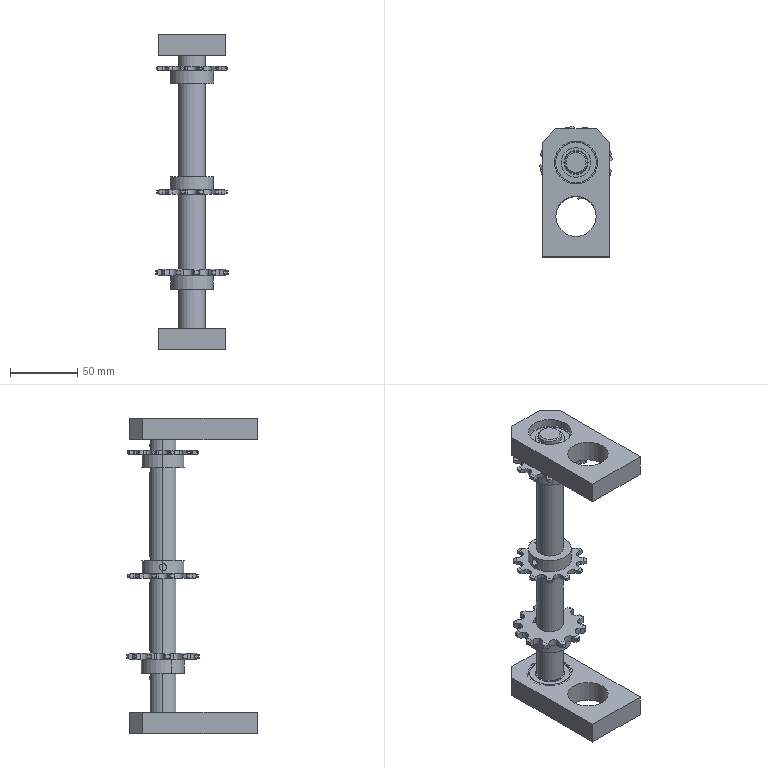Part | NX | features BREP 4, DATUM_CSYS 1, EXTRACT_DATUM_PLANE 1, EXTRUDE 1, SKETCH 1 | 8 solids | 440 faces | box 53.723 x 96.862 x 234.5 mm | volume 212399 mm3 | plane 197 | cylinder 151 | cone 76 | torus 16 | commonest cylinder face diameters 7.77 x51 53.9 x36 20 x11 6 x9 17 x8 22.033 x8